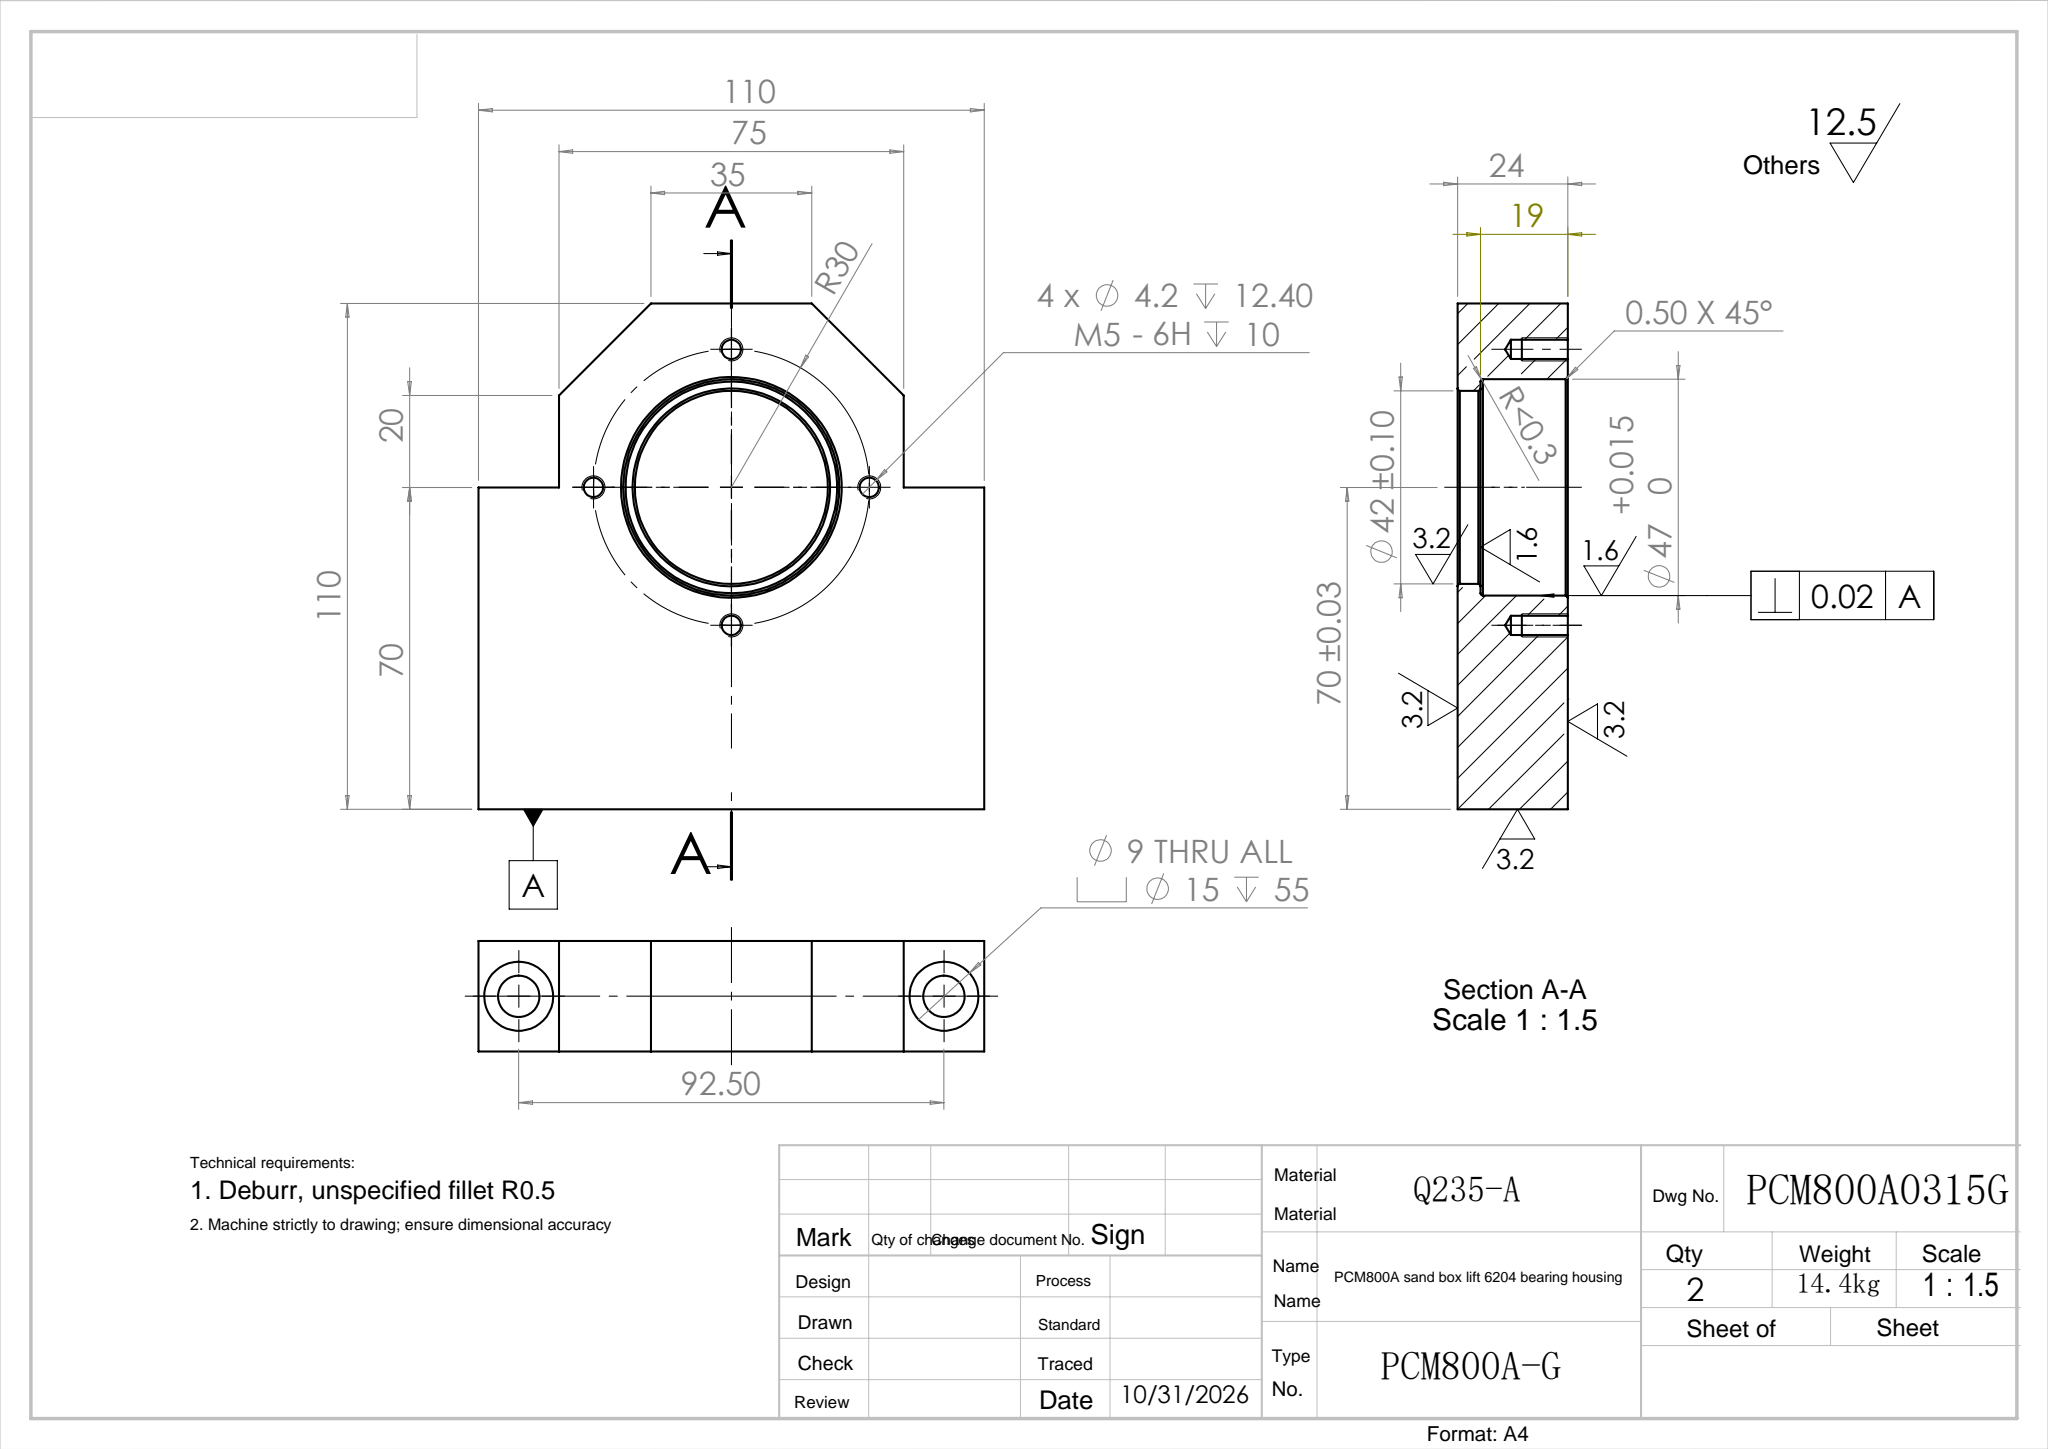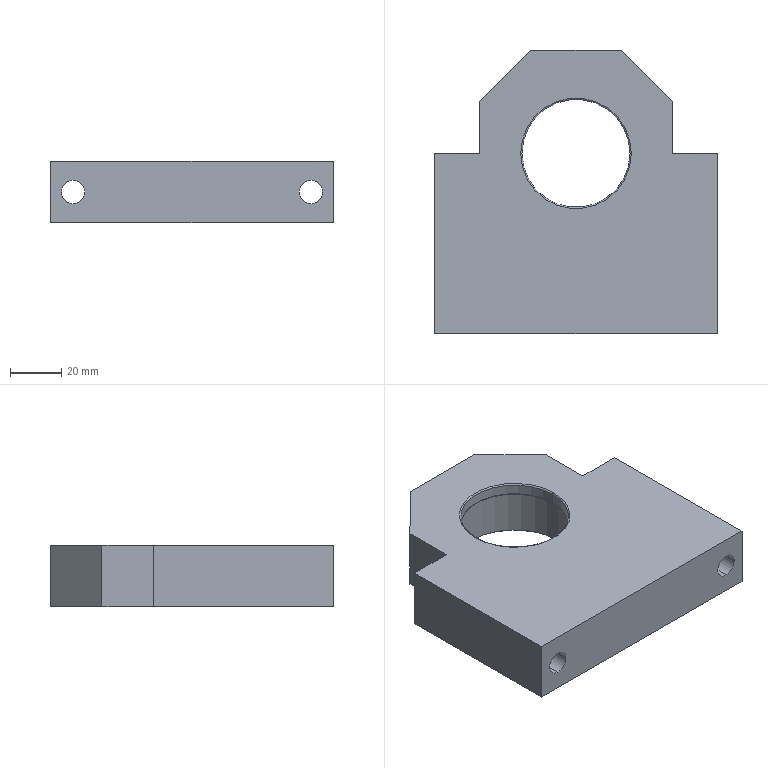Part | SolidWorks | features Cut 3, 3DProfileFeature 2, Chamfer 2, HoleWzd 2, Extrusion 1, Fillet 1 | 1 solid | 51 faces | box 110 x 110 x 24 mm | volume 185226 mm3 | cylinder 20 | plane 15 | cone 10 | torus 6 | commonest cylinder face diameters 4.2 x8 9 x4 15 x4 42 x2 47 x2